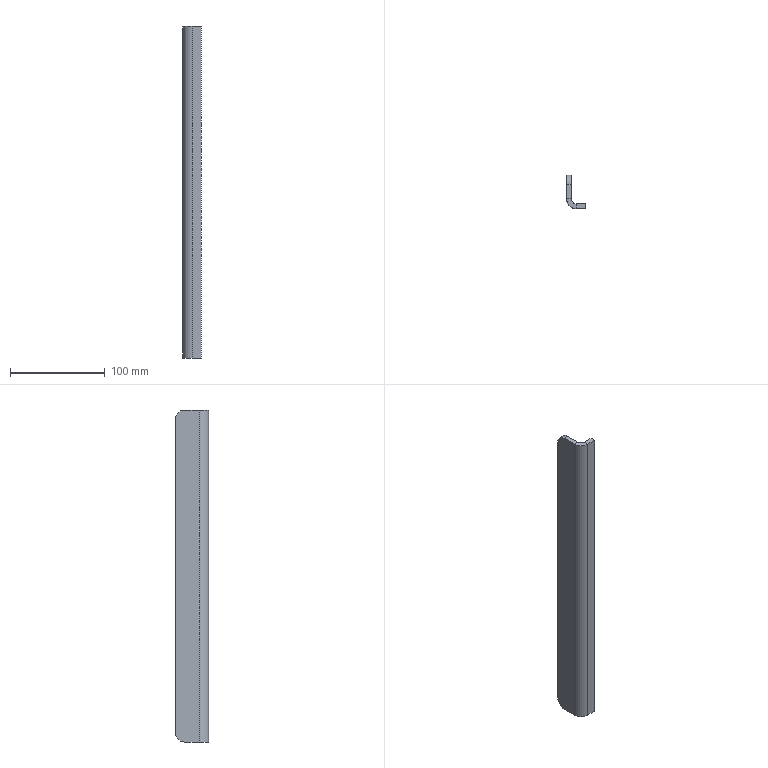Part | SolidWorks | features BaseBody 1, FlatPattern 1, SheetMetal 1, SolidToSheetMetal 1 | 1 solid | 16 faces | box 20 x 35 x 350 mm | volume 81652 mm3 | plane 12 | cylinder 4 | commonest cylinder face diameters 20 x3 10 x1
STEP:
#1=CARTESIAN_POINT('',(0.,25.,-175.));
#2=VERTEX_POINT('',#1);
#3=CARTESIAN_POINT('',(5.,25.,-175.));
#4=VERTEX_POINT('',#3);
#5=CARTESIAN_POINT('',(5.,25.,-175.));
#6=DIRECTION('',(1.,0.,0.));
#7=VECTOR('',#6,1000.);
#8=LINE('',#5,#7);
#9=EDGE_CURVE('',#2,#4,#8,.T.);
#10=ORIENTED_EDGE('',*,*,#9,.F.);
#11=CARTESIAN_POINT('',(0.,35.,-165.));
#12=VERTEX_POINT('',#11);
#13=CARTESIAN_POINT('',(0.,25.,-165.));
#14=DIRECTION('',(1.,0.,0.));
#15=DIRECTION('',(0.,0.,-1.));
#16=AXIS2_PLACEMENT_3D('',#13,#14,#15);
#17=CIRCLE('',#16,10.);
#18=EDGE_CURVE('',#2,#12,#17,.T.);
#19=ORIENTED_EDGE('',*,*,#18,.T.);
#20=CARTESIAN_POINT('',(5.,35.,-165.));
#21=VERTEX_POINT('',#20);
#22=CARTESIAN_POINT('',(5.,35.,-165.));
#23=DIRECTION('',(1.,0.,0.));
#24=VECTOR('',#23,1000.);
#25=LINE('',#22,#24);
#26=EDGE_CURVE('',#12,#21,#25,.T.);
#27=ORIENTED_EDGE('',*,*,#26,.T.);
#28=CARTESIAN_POINT('',(5.,25.,-165.));
#29=DIRECTION('',(1.,0.,0.));
#30=DIRECTION('',(0.,0.,-1.));
#31=AXIS2_PLACEMENT_3D('',#28,#29,#30);
#32=CIRCLE('',#31,10.);
#33=EDGE_CURVE('',#4,#21,#32,.T.);
#34=ORIENTED_EDGE('',*,*,#33,.F.);
#35=EDGE_LOOP('',(#10,#19,#27,#34));
#36=FACE_OUTER_BOUND('',#35,.T.);
#37=CARTESIAN_POINT('',(5.,25.,-165.));
#38=DIRECTION('',(-1.,0.,0.));
#39=DIRECTION('',(0.,0.,1.));
#40=AXIS2_PLACEMENT_3D('',#37,#38,#39);
#41=CYLINDRICAL_SURFACE('',#40,10.);
#42=ADVANCED_FACE('',(#36),#41,.T.);
#43=ORIENTED_EDGE('',*,*,#26,.F.);
#44=CARTESIAN_POINT('',(0.,35.,165.));
#45=VERTEX_POINT('',#44);
#46=CARTESIAN_POINT('',(0.,35.,-175.));
#47=DIRECTION('',(0.,0.,1.));
#48=VECTOR('',#47,1000.);
#49=LINE('',#46,#48);
#50=EDGE_CURVE('',#12,#45,#49,.T.);
#51=ORIENTED_EDGE('',*,*,#50,.T.);
#52=CARTESIAN_POINT('',(5.,35.,165.));
#53=VERTEX_POINT('',#52);
#54=CARTESIAN_POINT('',(5.,35.,165.));
#55=DIRECTION('',(1.,0.,0.));
#56=VECTOR('',#55,1000.);
#57=LINE('',#54,#56);
#58=EDGE_CURVE('',#45,#53,#57,.T.);
#59=ORIENTED_EDGE('',*,*,#58,.T.);
#60=CARTESIAN_POINT('',(5.,35.,-165.));
#61=DIRECTION('',(0.,0.,1.));
#62=VECTOR('',#61,1000.);
#63=LINE('',#60,#62);
#64=EDGE_CURVE('',#21,#53,#63,.T.);
#65=ORIENTED_EDGE('',*,*,#64,.F.);
#66=EDGE_LOOP('',(#43,#51,#59,#65));
#67=FACE_OUTER_BOUND('',#66,.T.);
#68=CARTESIAN_POINT('',(5.,35.,-165.));
#69=DIRECTION('',(0.,-1.,0.));
#70=DIRECTION('',(0.,0.,1.));
#71=AXIS2_PLACEMENT_3D('',#68,#69,#70);
#72=PLANE('',#71);
#73=ADVANCED_FACE('',(#67),#72,.F.);
#74=ORIENTED_EDGE('',*,*,#58,.F.);
#75=CARTESIAN_POINT('',(0.,25.,175.));
#76=VERTEX_POINT('',#75);
#77=CARTESIAN_POINT('',(0.,25.,165.));
#78=DIRECTION('',(1.,0.,0.));
#79=DIRECTION('',(0.,0.,-1.));
#80=AXIS2_PLACEMENT_3D('',#77,#78,#79);
#81=CIRCLE('',#80,10.);
#82=EDGE_CURVE('',#45,#76,#81,.T.);
#83=ORIENTED_EDGE('',*,*,#82,.T.);
#84=CARTESIAN_POINT('',(5.,25.,175.));
#85=VERTEX_POINT('',#84);
#86=CARTESIAN_POINT('',(5.,25.,175.));
#87=DIRECTION('',(1.,0.,0.));
#88=VECTOR('',#87,1000.);
#89=LINE('',#86,#88);
#90=EDGE_CURVE('',#76,#85,#89,.T.);
#91=ORIENTED_EDGE('',*,*,#90,.T.);
#92=CARTESIAN_POINT('',(5.,25.,165.));
#93=DIRECTION('',(1.,0.,0.));
#94=DIRECTION('',(0.,1.,0.));
#95=AXIS2_PLACEMENT_3D('',#92,#93,#94);
#96=CIRCLE('',#95,10.);
#97=EDGE_CURVE('',#53,#85,#96,.T.);
#98=ORIENTED_EDGE('',*,*,#97,.F.);
#99=EDGE_LOOP('',(#74,#83,#91,#98));
#100=FACE_OUTER_BOUND('',#99,.T.);
#101=CARTESIAN_POINT('',(5.,25.,165.));
#102=DIRECTION('',(-1.,0.,0.));
#103=DIRECTION('',(0.,0.,1.));
#104=AXIS2_PLACEMENT_3D('',#101,#102,#103);
#105=CYLINDRICAL_SURFACE('',#104,10.);
#106=ADVANCED_FACE('',(#100),#105,.T.);
#107=ORIENTED_EDGE('',*,*,#90,.F.);
#108=CARTESIAN_POINT('',(0.,10.,175.));
#109=VERTEX_POINT('',#108);
#110=CARTESIAN_POINT('',(0.,35.,175.));
#111=DIRECTION('',(0.,-1.,0.));
#112=VECTOR('',#111,1000.);
#113=LINE('',#110,#112);
#114=EDGE_CURVE('',#76,#109,#113,.T.);
#115=ORIENTED_EDGE('',*,*,#114,.T.);
#116=CARTESIAN_POINT('',(5.,10.,175.));
#117=VERTEX_POINT('',#116);
#118=CARTESIAN_POINT('',(5.,10.,175.));
#119=DIRECTION('',(1.,0.,0.));
#120=VECTOR('',#119,1000.);
#121=LINE('',#118,#120);
#122=EDGE_CURVE('',#109,#117,#121,.T.);
#123=ORIENTED_EDGE('',*,*,#122,.T.);
#124=CARTESIAN_POINT('',(5.,25.,175.));
#125=DIRECTION('',(0.,-1.,0.));
#126=VECTOR('',#125,1000.);
#127=LINE('',#124,#126);
#128=EDGE_CURVE('',#85,#117,#127,.T.);
#129=ORIENTED_EDGE('',*,*,#128,.F.);
#130=EDGE_LOOP('',(#107,#115,#123,#129));
#131=FACE_OUTER_BOUND('',#130,.T.);
#132=CARTESIAN_POINT('',(5.,25.,175.));
#133=DIRECTION('',(0.,0.,-1.));
#134=DIRECTION('',(0.,-1.,0.));
#135=AXIS2_PLACEMENT_3D('',#132,#133,#134);
#136=PLANE('',#135);
#137=ADVANCED_FACE('',(#131),#136,.F.);
#138=ORIENTED_EDGE('',*,*,#122,.F.);
#139=CARTESIAN_POINT('',(10.,0.,175.));
#140=VERTEX_POINT('',#139);
#141=CARTESIAN_POINT('',(10.,10.,175.));
#142=DIRECTION('',(0.,0.,-1.));
#143=DIRECTION('',(-1.,0.,0.));
#144=AXIS2_PLACEMENT_3D('',#141,#142,#143);
#145=CIRCLE('',#144,10.);
#146=EDGE_CURVE('',#140,#109,#145,.T.);
#147=ORIENTED_EDGE('',*,*,#146,.F.);
#148=CARTESIAN_POINT('',(10.,5.,175.));
#149=VERTEX_POINT('',#148);
#150=CARTESIAN_POINT('',(10.,5.,175.));
#151=DIRECTION('',(0.,1.,0.));
#152=VECTOR('',#151,1000.);
#153=LINE('',#150,#152);
#154=EDGE_CURVE('',#140,#149,#153,.T.);
#155=ORIENTED_EDGE('',*,*,#154,.T.);
#156=CARTESIAN_POINT('',(10.,10.,175.));
#157=DIRECTION('',(0.,0.,-1.));
#158=DIRECTION('',(0.,-1.,0.));
#159=AXIS2_PLACEMENT_3D('',#156,#157,#158);
#160=CIRCLE('',#159,5.);
#161=EDGE_CURVE('',#149,#117,#160,.T.);
#162=ORIENTED_EDGE('',*,*,#161,.T.);
#163=EDGE_LOOP('',(#138,#147,#155,#162));
#164=FACE_OUTER_BOUND('',#163,.T.);
#165=CARTESIAN_POINT('',(10.,10.,175.));
#166=DIRECTION('',(0.,0.,1.));
#167=DIRECTION('',(1.,0.,0.));
#168=AXIS2_PLACEMENT_3D('',#165,#166,#167);
#169=PLANE('',#168);
#170=ADVANCED_FACE('',(#164),#169,.T.);
#171=ORIENTED_EDGE('',*,*,#154,.F.);
#172=CARTESIAN_POINT('',(20.,0.,175.));
#173=VERTEX_POINT('',#172);
#174=CARTESIAN_POINT('',(0.,0.,175.));
#175=DIRECTION('',(1.,0.,0.));
#176=VECTOR('',#175,1000.);
#177=LINE('',#174,#176);
#178=EDGE_CURVE('',#140,#173,#177,.T.);
#179=ORIENTED_EDGE('',*,*,#178,.T.);
#180=CARTESIAN_POINT('',(20.,5.,175.));
#181=VERTEX_POINT('',#180);
#182=CARTESIAN_POINT('',(20.,5.,175.));
#183=DIRECTION('',(0.,1.,0.));
#184=VECTOR('',#183,1000.);
#185=LINE('',#182,#184);
#186=EDGE_CURVE('',#173,#181,#185,.T.);
#187=ORIENTED_EDGE('',*,*,#186,.T.);
#188=CARTESIAN_POINT('',(10.,5.,175.));
#189=DIRECTION('',(1.,0.,0.));
#190=VECTOR('',#189,1000.);
#191=LINE('',#188,#190);
#192=EDGE_CURVE('',#149,#181,#191,.T.);
#193=ORIENTED_EDGE('',*,*,#192,.F.);
#194=EDGE_LOOP('',(#171,#179,#187,#193));
#195=FACE_OUTER_BOUND('',#194,.T.);
#196=CARTESIAN_POINT('',(10.,5.,175.));
#197=DIRECTION('',(0.,0.,-1.));
#198=DIRECTION('',(1.,0.,0.));
#199=AXIS2_PLACEMENT_3D('',#196,#197,#198);
#200=PLANE('',#199);
#201=ADVANCED_FACE('',(#195),#200,.F.);
#202=ORIENTED_EDGE('',*,*,#186,.F.);
#203=CARTESIAN_POINT('',(20.,0.,-175.));
#204=VERTEX_POINT('',#203);
#205=CARTESIAN_POINT('',(20.,0.,-175.));
#206=DIRECTION('',(0.,0.,1.));
#207=VECTOR('',#206,1000.);
#208=LINE('',#205,#207);
#209=EDGE_CURVE('',#204,#173,#208,.T.);
#210=ORIENTED_EDGE('',*,*,#209,.F.);
#211=CARTESIAN_POINT('',(20.,5.,-175.));
#212=VERTEX_POINT('',#211);
#213=CARTESIAN_POINT('',(20.,5.,-175.));
#214=DIRECTION('',(0.,1.,0.));
#215=VECTOR('',#214,1000.);
#216=LINE('',#213,#215);
#217=EDGE_CURVE('',#204,#212,#216,.T.);
#218=ORIENTED_EDGE('',*,*,#217,.T.);
#219=CARTESIAN_POINT('',(20.,5.,-175.));
#220=DIRECTION('',(0.,0.,1.));
#221=VECTOR('',#220,1000.);
#222=LINE('',#219,#221);
#223=EDGE_CURVE('',#212,#181,#222,.T.);
#224=ORIENTED_EDGE('',*,*,#223,.T.);
#225=EDGE_LOOP('',(#202,#210,#218,#224));
#226=FACE_OUTER_BOUND('',#225,.T.);
#227=CARTESIAN_POINT('',(20.,5.,-175.));
#228=DIRECTION('',(1.,0.,0.));
#229=DIRECTION('',(0.,0.,1.));
#230=AXIS2_PLACEMENT_3D('',#227,#228,#229);
#231=PLANE('',#230);
#232=ADVANCED_FACE('',(#226),#231,.T.);
#233=ORIENTED_EDGE('',*,*,#217,.F.);
#234=CARTESIAN_POINT('',(10.,0.,-175.));
#235=VERTEX_POINT('',#234);
#236=CARTESIAN_POINT('',(0.,0.,-175.));
#237=DIRECTION('',(1.,0.,0.));
#238=VECTOR('',#237,1000.);
#239=LINE('',#236,#238);
#240=EDGE_CURVE('',#235,#204,#239,.T.);
#241=ORIENTED_EDGE('',*,*,#240,.F.);
#242=CARTESIAN_POINT('',(10.,5.,-175.));
#243=VERTEX_POINT('',#242);
#244=CARTESIAN_POINT('',(10.,5.,-175.));
#245=DIRECTION('',(0.,1.,0.));
#246=VECTOR('',#245,1000.);
#247=LINE('',#244,#246);
#248=EDGE_CURVE('',#235,#243,#247,.T.);
#249=ORIENTED_EDGE('',*,*,#248,.T.);
#250=CARTESIAN_POINT('',(10.,5.,-175.));
#251=DIRECTION('',(1.,0.,0.));
#252=VECTOR('',#251,1000.);
#253=LINE('',#250,#252);
#254=EDGE_CURVE('',#243,#212,#253,.T.);
#255=ORIENTED_EDGE('',*,*,#254,.T.);
#256=EDGE_LOOP('',(#233,#241,#249,#255));
#257=FACE_OUTER_BOUND('',#256,.T.);
#258=CARTESIAN_POINT('',(10.,5.,-175.));
#259=DIRECTION('',(0.,0.,-1.));
#260=DIRECTION('',(1.,0.,0.));
#261=AXIS2_PLACEMENT_3D('',#258,#259,#260);
#262=PLANE('',#261);
#263=ADVANCED_FACE('',(#257),#262,.T.);
#264=ORIENTED_EDGE('',*,*,#248,.F.);
#265=CARTESIAN_POINT('',(0.,10.,-175.));
#266=VERTEX_POINT('',#265);
#267=CARTESIAN_POINT('',(10.,10.,-175.));
#268=DIRECTION('',(0.,0.,-1.));
#269=DIRECTION('',(-1.,0.,0.));
#270=AXIS2_PLACEMENT_3D('',#267,#268,#269);
#271=CIRCLE('',#270,10.);
#272=EDGE_CURVE('',#235,#266,#271,.T.);
#273=ORIENTED_EDGE('',*,*,#272,.T.);
#274=CARTESIAN_POINT('',(5.,10.,-175.));
#275=VERTEX_POINT('',#274);
#276=CARTESIAN_POINT('',(5.,10.,-175.));
#277=DIRECTION('',(1.,0.,0.));
#278=VECTOR('',#277,1000.);
#279=LINE('',#276,#278);
#280=EDGE_CURVE('',#266,#275,#279,.T.);
#281=ORIENTED_EDGE('',*,*,#280,.T.);
#282=CARTESIAN_POINT('',(10.,10.,-175.));
#283=DIRECTION('',(0.,0.,-1.));
#284=DIRECTION('',(0.,-1.,0.));
#285=AXIS2_PLACEMENT_3D('',#282,#283,#284);
#286=CIRCLE('',#285,5.);
#287=EDGE_CURVE('',#243,#275,#286,.T.);
#288=ORIENTED_EDGE('',*,*,#287,.F.);
#289=EDGE_LOOP('',(#264,#273,#281,#288));
#290=FACE_OUTER_BOUND('',#289,.T.);
#291=CARTESIAN_POINT('',(10.,10.,-175.));
#292=DIRECTION('',(0.,0.,1.));
#293=DIRECTION('',(1.,0.,0.));
#294=AXIS2_PLACEMENT_3D('',#291,#292,#293);
#295=PLANE('',#294);
#296=ADVANCED_FACE('',(#290),#295,.F.);
#297=CARTESIAN_POINT('',(0.,35.,-175.));
#298=DIRECTION('',(0.,-1.,0.));
#299=VECTOR('',#298,1000.);
#300=LINE('',#297,#299);
#301=EDGE_CURVE('',#2,#266,#300,.T.);
#302=ORIENTED_EDGE('',*,*,#301,.F.);
#303=ORIENTED_EDGE('',*,*,#9,.T.);
#304=CARTESIAN_POINT('',(5.,25.,-175.));
#305=DIRECTION('',(0.,-1.,0.));
#306=VECTOR('',#305,1000.);
#307=LINE('',#304,#306);
#308=EDGE_CURVE('',#4,#275,#307,.T.);
#309=ORIENTED_EDGE('',*,*,#308,.T.);
#310=ORIENTED_EDGE('',*,*,#280,.F.);
#311=EDGE_LOOP('',(#302,#303,#309,#310));
#312=FACE_OUTER_BOUND('',#311,.T.);
#313=CARTESIAN_POINT('',(5.,25.,-175.));
#314=DIRECTION('',(0.,0.,-1.));
#315=DIRECTION('',(0.,-1.,0.));
#316=AXIS2_PLACEMENT_3D('',#313,#314,#315);
#317=PLANE('',#316);
#318=ADVANCED_FACE('',(#312),#317,.T.);
#319=ORIENTED_EDGE('',*,*,#287,.T.);
#320=CARTESIAN_POINT('',(5.,10.,-175.));
#321=DIRECTION('',(0.,0.,1.));
#322=VECTOR('',#321,1000.);
#323=LINE('',#320,#322);
#324=EDGE_CURVE('',#275,#117,#323,.T.);
#325=ORIENTED_EDGE('',*,*,#324,.T.);
#326=ORIENTED_EDGE('',*,*,#161,.F.);
#327=CARTESIAN_POINT('',(10.,5.,-175.));
#328=DIRECTION('',(0.,0.,1.));
#329=VECTOR('',#328,1000.);
#330=LINE('',#327,#329);
#331=EDGE_CURVE('',#243,#149,#330,.T.);
#332=ORIENTED_EDGE('',*,*,#331,.F.);
#333=EDGE_LOOP('',(#319,#325,#326,#332));
#334=FACE_OUTER_BOUND('',#333,.T.);
#335=CARTESIAN_POINT('',(10.,10.,-175.));
#336=DIRECTION('',(0.,0.,-1.));
#337=DIRECTION('',(0.,-1.,0.));
#338=AXIS2_PLACEMENT_3D('',#335,#336,#337);
#339=CYLINDRICAL_SURFACE('',#338,5.);
#340=ADVANCED_FACE('',(#334),#339,.F.);
#341=ORIENTED_EDGE('',*,*,#331,.T.);
#342=ORIENTED_EDGE('',*,*,#192,.T.);
#343=ORIENTED_EDGE('',*,*,#223,.F.);
#344=ORIENTED_EDGE('',*,*,#254,.F.);
#345=EDGE_LOOP('',(#341,#342,#343,#344));
#346=FACE_OUTER_BOUND('',#345,.T.);
#347=CARTESIAN_POINT('',(0.,5.,-175.));
#348=DIRECTION('',(0.,-1.,0.));
#349=DIRECTION('',(0.,0.,-1.));
#350=AXIS2_PLACEMENT_3D('',#347,#348,#349);
#351=PLANE('',#350);
#352=ADVANCED_FACE('',(#346),#351,.F.);
#353=ORIENTED_EDGE('',*,*,#128,.T.);
#354=ORIENTED_EDGE('',*,*,#324,.F.);
#355=ORIENTED_EDGE('',*,*,#308,.F.);
#356=ORIENTED_EDGE('',*,*,#33,.T.);
#357=ORIENTED_EDGE('',*,*,#64,.T.);
#358=ORIENTED_EDGE('',*,*,#97,.T.);
#359=EDGE_LOOP('',(#353,#354,#355,#356,#357,#358));
#360=FACE_OUTER_BOUND('',#359,.T.);
#361=CARTESIAN_POINT('',(5.,35.,-175.));
#362=DIRECTION('',(-1.,0.,0.));
#363=DIRECTION('',(0.,0.,1.));
#364=AXIS2_PLACEMENT_3D('',#361,#362,#363);
#365=PLANE('',#364);
#366=ADVANCED_FACE('',(#360),#365,.F.);
#367=ORIENTED_EDGE('',*,*,#272,.F.);
#368=CARTESIAN_POINT('',(10.,0.,-175.));
#369=DIRECTION('',(0.,0.,1.));
#370=VECTOR('',#369,1000.);
#371=LINE('',#368,#370);
#372=EDGE_CURVE('',#235,#140,#371,.T.);
#373=ORIENTED_EDGE('',*,*,#372,.T.);
#374=ORIENTED_EDGE('',*,*,#146,.T.);
#375=CARTESIAN_POINT('',(0.,10.,-175.));
#376=DIRECTION('',(0.,0.,1.));
#377=VECTOR('',#376,1000.);
#378=LINE('',#375,#377);
#379=EDGE_CURVE('',#266,#109,#378,.T.);
#380=ORIENTED_EDGE('',*,*,#379,.F.);
#381=EDGE_LOOP('',(#367,#373,#374,#380));
#382=FACE_OUTER_BOUND('',#381,.T.);
#383=CARTESIAN_POINT('',(10.,10.,-175.));
#384=DIRECTION('',(0.,0.,-1.));
#385=DIRECTION('',(0.,-1.,0.));
#386=AXIS2_PLACEMENT_3D('',#383,#384,#385);
#387=CYLINDRICAL_SURFACE('',#386,10.);
#388=ADVANCED_FACE('',(#382),#387,.T.);
#389=ORIENTED_EDGE('',*,*,#372,.F.);
#390=ORIENTED_EDGE('',*,*,#240,.T.);
#391=ORIENTED_EDGE('',*,*,#209,.T.);
#392=ORIENTED_EDGE('',*,*,#178,.F.);
#393=EDGE_LOOP('',(#389,#390,#391,#392));
#394=FACE_OUTER_BOUND('',#393,.T.);
#395=CARTESIAN_POINT('',(0.,0.,-175.));
#396=DIRECTION('',(0.,-1.,0.));
#397=DIRECTION('',(0.,0.,-1.));
#398=AXIS2_PLACEMENT_3D('',#395,#396,#397);
#399=PLANE('',#398);
#400=ADVANCED_FACE('',(#394),#399,.T.);
#401=ORIENTED_EDGE('',*,*,#114,.F.);
#402=ORIENTED_EDGE('',*,*,#82,.F.);
#403=ORIENTED_EDGE('',*,*,#50,.F.);
#404=ORIENTED_EDGE('',*,*,#18,.F.);
#405=ORIENTED_EDGE('',*,*,#301,.T.);
#406=ORIENTED_EDGE('',*,*,#379,.T.);
#407=EDGE_LOOP('',(#401,#402,#403,#404,#405,#406));
#408=FACE_OUTER_BOUND('',#407,.T.);
#409=CARTESIAN_POINT('',(0.,35.,-175.));
#410=DIRECTION('',(-1.,0.,0.));
#411=DIRECTION('',(0.,0.,1.));
#412=AXIS2_PLACEMENT_3D('',#409,#410,#411);
#413=PLANE('',#412);
#414=ADVANCED_FACE('',(#408),#413,.T.);
#415=CLOSED_SHELL('',(#42,#73,#106,#137,#170,#201,#232,#263,#296,#318,#340,#352,#366,#388,#400,#414));
#416=MANIFOLD_SOLID_BREP('',#415);
#417=CARTESIAN_POINT('',(0.,0.,0.));
#418=DIRECTION('',(0.,0.,1.));
#419=DIRECTION('',(1.,0.,0.));
#420=AXIS2_PLACEMENT_3D('',#417,#418,#419);
#421=(LENGTH_UNIT()NAMED_UNIT(*)SI_UNIT(.MILLI.,.METRE.));
#422=UNCERTAINTY_MEASURE_WITH_UNIT(LENGTH_MEASURE(0.00001),#421,'','');
#423=(NAMED_UNIT(*)PLANE_ANGLE_UNIT()SI_UNIT($,.RADIAN.));
#424=(NAMED_UNIT(*)SI_UNIT($,.STERADIAN.)SOLID_ANGLE_UNIT());
#425=(GEOMETRIC_REPRESENTATION_CONTEXT(3)GLOBAL_UNCERTAINTY_ASSIGNED_CONTEXT((#422))GLOBAL_UNIT_ASSIGNED_CONTEXT((#421,#423,#424))REPRESENTATION_CONTEXT('',''));
#426=ADVANCED_BREP_SHAPE_REPRESENTATION('',(#416,#420),#425);